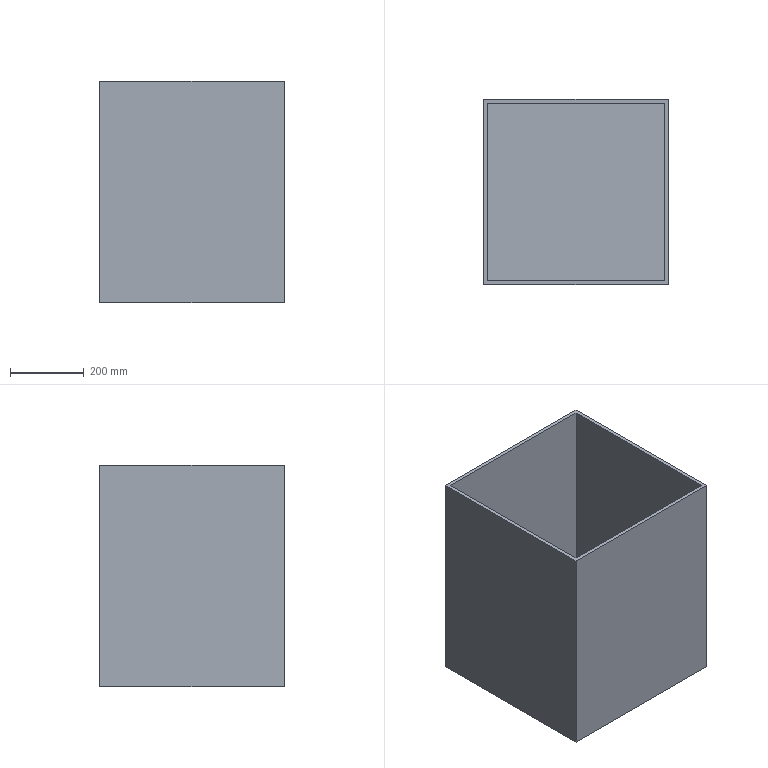Part | SolidWorks | features Extrusion 1, Shell 1 | 1 solid | 11 faces | box 500 x 500 x 600 mm | volume 14064000 mm3 | plane 11
STEP:
#1=CARTESIAN_POINT('',(0.,500.,600.));
#2=VERTEX_POINT('',#1);
#3=CARTESIAN_POINT('',(0.,0.,600.));
#4=VERTEX_POINT('',#3);
#5=CARTESIAN_POINT('',(0.,0.,600.));
#6=DIRECTION('',(0.,-1.,0.));
#7=VECTOR('',#6,1000.);
#8=LINE('',#5,#7);
#9=EDGE_CURVE('',#2,#4,#8,.T.);
#10=ORIENTED_EDGE('',*,*,#9,.T.);
#11=CARTESIAN_POINT('',(500.,0.,600.));
#12=VERTEX_POINT('',#11);
#13=CARTESIAN_POINT('',(0.,0.,600.));
#14=DIRECTION('',(1.,0.,0.));
#15=VECTOR('',#14,1000.);
#16=LINE('',#13,#15);
#17=EDGE_CURVE('',#4,#12,#16,.T.);
#18=ORIENTED_EDGE('',*,*,#17,.T.);
#19=CARTESIAN_POINT('',(500.,500.,600.));
#20=VERTEX_POINT('',#19);
#21=CARTESIAN_POINT('',(500.,0.,600.));
#22=DIRECTION('',(0.,1.,0.));
#23=VECTOR('',#22,1000.);
#24=LINE('',#21,#23);
#25=EDGE_CURVE('',#12,#20,#24,.T.);
#26=ORIENTED_EDGE('',*,*,#25,.T.);
#27=CARTESIAN_POINT('',(0.,500.,600.));
#28=DIRECTION('',(-1.,0.,0.));
#29=VECTOR('',#28,1000.);
#30=LINE('',#27,#29);
#31=EDGE_CURVE('',#20,#2,#30,.T.);
#32=ORIENTED_EDGE('',*,*,#31,.T.);
#33=EDGE_LOOP('',(#10,#18,#26,#32));
#34=FACE_OUTER_BOUND('',#33,.T.);
#35=CARTESIAN_POINT('',(10.,490.,600.));
#36=VERTEX_POINT('',#35);
#37=CARTESIAN_POINT('',(10.,10.,600.));
#38=VERTEX_POINT('',#37);
#39=CARTESIAN_POINT('',(10.,0.,600.));
#40=DIRECTION('',(0.,-1.,0.));
#41=VECTOR('',#40,1000.);
#42=LINE('',#39,#41);
#43=EDGE_CURVE('',#36,#38,#42,.T.);
#44=ORIENTED_EDGE('',*,*,#43,.F.);
#45=CARTESIAN_POINT('',(490.,490.,600.));
#46=VERTEX_POINT('',#45);
#47=CARTESIAN_POINT('',(0.,490.,600.));
#48=DIRECTION('',(-1.,0.,0.));
#49=VECTOR('',#48,1000.);
#50=LINE('',#47,#49);
#51=EDGE_CURVE('',#46,#36,#50,.T.);
#52=ORIENTED_EDGE('',*,*,#51,.F.);
#53=CARTESIAN_POINT('',(490.,10.,600.));
#54=VERTEX_POINT('',#53);
#55=CARTESIAN_POINT('',(490.,0.,600.));
#56=DIRECTION('',(0.,1.,0.));
#57=VECTOR('',#56,1000.);
#58=LINE('',#55,#57);
#59=EDGE_CURVE('',#54,#46,#58,.T.);
#60=ORIENTED_EDGE('',*,*,#59,.F.);
#61=CARTESIAN_POINT('',(0.,10.,600.));
#62=DIRECTION('',(1.,0.,0.));
#63=VECTOR('',#62,1000.);
#64=LINE('',#61,#63);
#65=EDGE_CURVE('',#38,#54,#64,.T.);
#66=ORIENTED_EDGE('',*,*,#65,.F.);
#67=EDGE_LOOP('',(#44,#52,#60,#66));
#68=FACE_BOUND('',#67,.T.);
#69=CARTESIAN_POINT('',(0.,0.,600.));
#70=DIRECTION('',(0.,0.,-1.));
#71=DIRECTION('',(-1.,0.,0.));
#72=AXIS2_PLACEMENT_3D('',#69,#70,#71);
#73=PLANE('',#72);
#74=ADVANCED_FACE('',(#34,#68),#73,.F.);
#75=CARTESIAN_POINT('',(0.,500.,0.));
#76=VERTEX_POINT('',#75);
#77=CARTESIAN_POINT('',(0.,0.,0.));
#78=VERTEX_POINT('',#77);
#79=CARTESIAN_POINT('',(0.,0.,0.));
#80=DIRECTION('',(0.,-1.,0.));
#81=VECTOR('',#80,1000.);
#82=LINE('',#79,#81);
#83=EDGE_CURVE('',#76,#78,#82,.T.);
#84=ORIENTED_EDGE('',*,*,#83,.T.);
#85=CARTESIAN_POINT('',(0.,0.,600.));
#86=DIRECTION('',(0.,0.,-1.));
#87=VECTOR('',#86,1000.);
#88=LINE('',#85,#87);
#89=EDGE_CURVE('',#4,#78,#88,.T.);
#90=ORIENTED_EDGE('',*,*,#89,.F.);
#91=ORIENTED_EDGE('',*,*,#9,.F.);
#92=CARTESIAN_POINT('',(0.,500.,600.));
#93=DIRECTION('',(0.,0.,-1.));
#94=VECTOR('',#93,1000.);
#95=LINE('',#92,#94);
#96=EDGE_CURVE('',#2,#76,#95,.T.);
#97=ORIENTED_EDGE('',*,*,#96,.T.);
#98=EDGE_LOOP('',(#84,#90,#91,#97));
#99=FACE_OUTER_BOUND('',#98,.T.);
#100=CARTESIAN_POINT('',(0.,0.,600.));
#101=DIRECTION('',(1.,0.,0.));
#102=DIRECTION('',(0.,0.,-1.));
#103=AXIS2_PLACEMENT_3D('',#100,#101,#102);
#104=PLANE('',#103);
#105=ADVANCED_FACE('',(#99),#104,.F.);
#106=CARTESIAN_POINT('',(500.,0.,0.));
#107=VERTEX_POINT('',#106);
#108=CARTESIAN_POINT('',(0.,0.,0.));
#109=DIRECTION('',(1.,0.,0.));
#110=VECTOR('',#109,1000.);
#111=LINE('',#108,#110);
#112=EDGE_CURVE('',#78,#107,#111,.T.);
#113=ORIENTED_EDGE('',*,*,#112,.T.);
#114=CARTESIAN_POINT('',(500.,0.,600.));
#115=DIRECTION('',(0.,0.,-1.));
#116=VECTOR('',#115,1000.);
#117=LINE('',#114,#116);
#118=EDGE_CURVE('',#12,#107,#117,.T.);
#119=ORIENTED_EDGE('',*,*,#118,.F.);
#120=ORIENTED_EDGE('',*,*,#17,.F.);
#121=ORIENTED_EDGE('',*,*,#89,.T.);
#122=EDGE_LOOP('',(#113,#119,#120,#121));
#123=FACE_OUTER_BOUND('',#122,.T.);
#124=CARTESIAN_POINT('',(0.,0.,600.));
#125=DIRECTION('',(0.,1.,0.));
#126=DIRECTION('',(0.,0.,1.));
#127=AXIS2_PLACEMENT_3D('',#124,#125,#126);
#128=PLANE('',#127);
#129=ADVANCED_FACE('',(#123),#128,.F.);
#130=CARTESIAN_POINT('',(500.,500.,0.));
#131=VERTEX_POINT('',#130);
#132=CARTESIAN_POINT('',(500.,0.,0.));
#133=DIRECTION('',(0.,1.,0.));
#134=VECTOR('',#133,1000.);
#135=LINE('',#132,#134);
#136=EDGE_CURVE('',#107,#131,#135,.T.);
#137=ORIENTED_EDGE('',*,*,#136,.T.);
#138=CARTESIAN_POINT('',(500.,500.,600.));
#139=DIRECTION('',(0.,0.,-1.));
#140=VECTOR('',#139,1000.);
#141=LINE('',#138,#140);
#142=EDGE_CURVE('',#20,#131,#141,.T.);
#143=ORIENTED_EDGE('',*,*,#142,.F.);
#144=ORIENTED_EDGE('',*,*,#25,.F.);
#145=ORIENTED_EDGE('',*,*,#118,.T.);
#146=EDGE_LOOP('',(#137,#143,#144,#145));
#147=FACE_OUTER_BOUND('',#146,.T.);
#148=CARTESIAN_POINT('',(500.,0.,600.));
#149=DIRECTION('',(-1.,0.,0.));
#150=DIRECTION('',(0.,0.,1.));
#151=AXIS2_PLACEMENT_3D('',#148,#149,#150);
#152=PLANE('',#151);
#153=ADVANCED_FACE('',(#147),#152,.F.);
#154=CARTESIAN_POINT('',(0.,500.,0.));
#155=DIRECTION('',(-1.,0.,0.));
#156=VECTOR('',#155,1000.);
#157=LINE('',#154,#156);
#158=EDGE_CURVE('',#131,#76,#157,.T.);
#159=ORIENTED_EDGE('',*,*,#158,.T.);
#160=ORIENTED_EDGE('',*,*,#96,.F.);
#161=ORIENTED_EDGE('',*,*,#31,.F.);
#162=ORIENTED_EDGE('',*,*,#142,.T.);
#163=EDGE_LOOP('',(#159,#160,#161,#162));
#164=FACE_OUTER_BOUND('',#163,.T.);
#165=CARTESIAN_POINT('',(0.,500.,600.));
#166=DIRECTION('',(0.,-1.,0.));
#167=DIRECTION('',(0.,0.,-1.));
#168=AXIS2_PLACEMENT_3D('',#165,#166,#167);
#169=PLANE('',#168);
#170=ADVANCED_FACE('',(#164),#169,.F.);
#171=ORIENTED_EDGE('',*,*,#83,.F.);
#172=ORIENTED_EDGE('',*,*,#158,.F.);
#173=ORIENTED_EDGE('',*,*,#136,.F.);
#174=ORIENTED_EDGE('',*,*,#112,.F.);
#175=EDGE_LOOP('',(#171,#172,#173,#174));
#176=FACE_OUTER_BOUND('',#175,.T.);
#177=CARTESIAN_POINT('',(0.,0.,0.));
#178=DIRECTION('',(0.,0.,-1.));
#179=DIRECTION('',(-1.,0.,0.));
#180=AXIS2_PLACEMENT_3D('',#177,#178,#179);
#181=PLANE('',#180);
#182=ADVANCED_FACE('',(#176),#181,.T.);
#183=CARTESIAN_POINT('',(10.,490.,10.));
#184=VERTEX_POINT('',#183);
#185=CARTESIAN_POINT('',(10.,10.,10.));
#186=VERTEX_POINT('',#185);
#187=CARTESIAN_POINT('',(10.,0.,10.));
#188=DIRECTION('',(0.,-1.,0.));
#189=VECTOR('',#188,1000.);
#190=LINE('',#187,#189);
#191=EDGE_CURVE('',#184,#186,#190,.T.);
#192=ORIENTED_EDGE('',*,*,#191,.F.);
#193=CARTESIAN_POINT('',(10.,490.,600.));
#194=DIRECTION('',(0.,0.,-1.));
#195=VECTOR('',#194,1000.);
#196=LINE('',#193,#195);
#197=EDGE_CURVE('',#36,#184,#196,.T.);
#198=ORIENTED_EDGE('',*,*,#197,.F.);
#199=ORIENTED_EDGE('',*,*,#43,.T.);
#200=CARTESIAN_POINT('',(10.,10.,600.));
#201=DIRECTION('',(0.,0.,-1.));
#202=VECTOR('',#201,1000.);
#203=LINE('',#200,#202);
#204=EDGE_CURVE('',#38,#186,#203,.T.);
#205=ORIENTED_EDGE('',*,*,#204,.T.);
#206=EDGE_LOOP('',(#192,#198,#199,#205));
#207=FACE_OUTER_BOUND('',#206,.T.);
#208=CARTESIAN_POINT('',(10.,0.,600.));
#209=DIRECTION('',(1.,0.,0.));
#210=DIRECTION('',(0.,0.,-1.));
#211=AXIS2_PLACEMENT_3D('',#208,#209,#210);
#212=PLANE('',#211);
#213=ADVANCED_FACE('',(#207),#212,.T.);
#214=CARTESIAN_POINT('',(490.,10.,10.));
#215=VERTEX_POINT('',#214);
#216=CARTESIAN_POINT('',(0.,10.,10.));
#217=DIRECTION('',(1.,0.,0.));
#218=VECTOR('',#217,1000.);
#219=LINE('',#216,#218);
#220=EDGE_CURVE('',#186,#215,#219,.T.);
#221=ORIENTED_EDGE('',*,*,#220,.F.);
#222=ORIENTED_EDGE('',*,*,#204,.F.);
#223=ORIENTED_EDGE('',*,*,#65,.T.);
#224=CARTESIAN_POINT('',(490.,10.,600.));
#225=DIRECTION('',(0.,0.,-1.));
#226=VECTOR('',#225,1000.);
#227=LINE('',#224,#226);
#228=EDGE_CURVE('',#54,#215,#227,.T.);
#229=ORIENTED_EDGE('',*,*,#228,.T.);
#230=EDGE_LOOP('',(#221,#222,#223,#229));
#231=FACE_OUTER_BOUND('',#230,.T.);
#232=CARTESIAN_POINT('',(0.,10.,600.));
#233=DIRECTION('',(0.,1.,0.));
#234=DIRECTION('',(0.,0.,1.));
#235=AXIS2_PLACEMENT_3D('',#232,#233,#234);
#236=PLANE('',#235);
#237=ADVANCED_FACE('',(#231),#236,.T.);
#238=CARTESIAN_POINT('',(490.,490.,10.));
#239=VERTEX_POINT('',#238);
#240=CARTESIAN_POINT('',(490.,0.,10.));
#241=DIRECTION('',(0.,1.,0.));
#242=VECTOR('',#241,1000.);
#243=LINE('',#240,#242);
#244=EDGE_CURVE('',#215,#239,#243,.T.);
#245=ORIENTED_EDGE('',*,*,#244,.F.);
#246=ORIENTED_EDGE('',*,*,#228,.F.);
#247=ORIENTED_EDGE('',*,*,#59,.T.);
#248=CARTESIAN_POINT('',(490.,490.,600.));
#249=DIRECTION('',(0.,0.,-1.));
#250=VECTOR('',#249,1000.);
#251=LINE('',#248,#250);
#252=EDGE_CURVE('',#46,#239,#251,.T.);
#253=ORIENTED_EDGE('',*,*,#252,.T.);
#254=EDGE_LOOP('',(#245,#246,#247,#253));
#255=FACE_OUTER_BOUND('',#254,.T.);
#256=CARTESIAN_POINT('',(490.,0.,600.));
#257=DIRECTION('',(-1.,0.,0.));
#258=DIRECTION('',(0.,0.,1.));
#259=AXIS2_PLACEMENT_3D('',#256,#257,#258);
#260=PLANE('',#259);
#261=ADVANCED_FACE('',(#255),#260,.T.);
#262=CARTESIAN_POINT('',(0.,490.,10.));
#263=DIRECTION('',(-1.,0.,0.));
#264=VECTOR('',#263,1000.);
#265=LINE('',#262,#264);
#266=EDGE_CURVE('',#239,#184,#265,.T.);
#267=ORIENTED_EDGE('',*,*,#266,.F.);
#268=ORIENTED_EDGE('',*,*,#252,.F.);
#269=ORIENTED_EDGE('',*,*,#51,.T.);
#270=ORIENTED_EDGE('',*,*,#197,.T.);
#271=EDGE_LOOP('',(#267,#268,#269,#270));
#272=FACE_OUTER_BOUND('',#271,.T.);
#273=CARTESIAN_POINT('',(0.,490.,600.));
#274=DIRECTION('',(0.,-1.,0.));
#275=DIRECTION('',(0.,0.,-1.));
#276=AXIS2_PLACEMENT_3D('',#273,#274,#275);
#277=PLANE('',#276);
#278=ADVANCED_FACE('',(#272),#277,.T.);
#279=ORIENTED_EDGE('',*,*,#191,.T.);
#280=ORIENTED_EDGE('',*,*,#220,.T.);
#281=ORIENTED_EDGE('',*,*,#244,.T.);
#282=ORIENTED_EDGE('',*,*,#266,.T.);
#283=EDGE_LOOP('',(#279,#280,#281,#282));
#284=FACE_OUTER_BOUND('',#283,.T.);
#285=CARTESIAN_POINT('',(0.,0.,10.));
#286=DIRECTION('',(0.,0.,-1.));
#287=DIRECTION('',(-1.,0.,0.));
#288=AXIS2_PLACEMENT_3D('',#285,#286,#287);
#289=PLANE('',#288);
#290=ADVANCED_FACE('',(#284),#289,.F.);
#291=CLOSED_SHELL('',(#74,#105,#129,#153,#170,#182,#213,#237,#261,#278,#290));
#292=MANIFOLD_SOLID_BREP('',#291);
#293=CARTESIAN_POINT('',(0.,0.,0.));
#294=DIRECTION('',(0.,0.,1.));
#295=DIRECTION('',(1.,0.,0.));
#296=AXIS2_PLACEMENT_3D('',#293,#294,#295);
#297=(LENGTH_UNIT()NAMED_UNIT(*)SI_UNIT(.MILLI.,.METRE.));
#298=UNCERTAINTY_MEASURE_WITH_UNIT(LENGTH_MEASURE(0.00001),#297,'','');
#299=(NAMED_UNIT(*)PLANE_ANGLE_UNIT()SI_UNIT($,.RADIAN.));
#300=(NAMED_UNIT(*)SI_UNIT($,.STERADIAN.)SOLID_ANGLE_UNIT());
#301=(GEOMETRIC_REPRESENTATION_CONTEXT(3)GLOBAL_UNCERTAINTY_ASSIGNED_CONTEXT((#298))GLOBAL_UNIT_ASSIGNED_CONTEXT((#297,#299,#300))REPRESENTATION_CONTEXT('',''));
#302=ADVANCED_BREP_SHAPE_REPRESENTATION('',(#292,#296),#301);